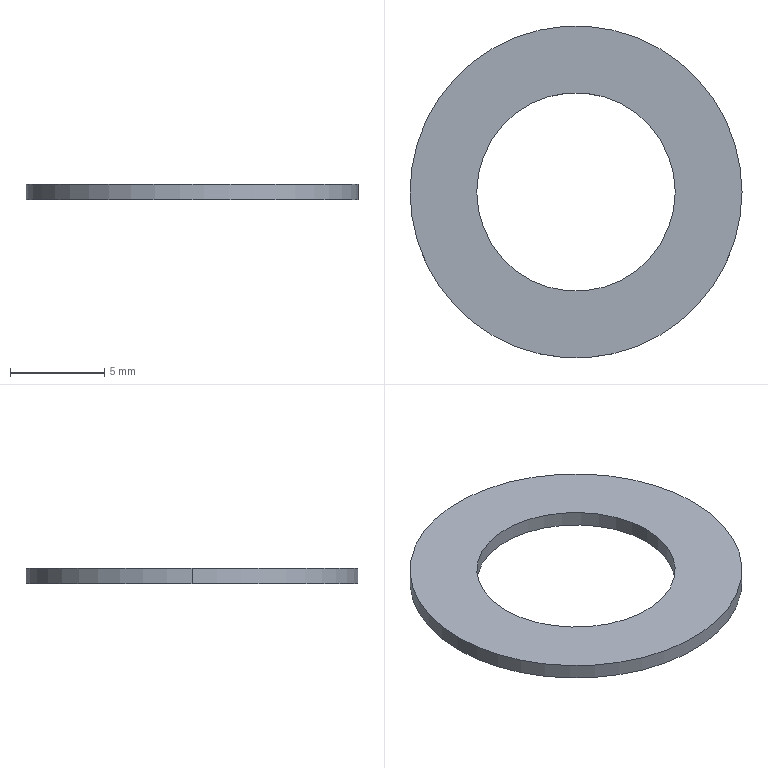Part | STEP file | 1 solid | 6 faces | box 17.57 x 17.57 x 0.8 mm | volume 124.693 mm3 | cylinder 4 | plane 2 | commonest cylinder face diameters 10.5 x2 17.57 x2
STEP:
#1=CARTESIAN_POINT('',(-5.25,0.,0.8));
#2=VERTEX_POINT('',#1);
#3=CARTESIAN_POINT('',(5.25,0.,0.8));
#4=VERTEX_POINT('',#3);
#5=CARTESIAN_POINT('',(0.,0.,0.8));
#6=DIRECTION('',(0.,0.,1.));
#7=DIRECTION('',(1.,0.,0.));
#8=AXIS2_PLACEMENT_3D('',#5,#6,#7);
#9=CIRCLE('',#8,5.25);
#10=EDGE_CURVE('',#2,#4,#9,.T.);
#11=ORIENTED_EDGE('',*,*,#10,.T.);
#12=CARTESIAN_POINT('',(5.25,0.,0.));
#13=VERTEX_POINT('',#12);
#14=CARTESIAN_POINT('',(5.25,0.,0.8));
#15=DIRECTION('',(0.,0.,-1.));
#16=VECTOR('',#15,1000.);
#17=LINE('',#14,#16);
#18=EDGE_CURVE('',#4,#13,#17,.T.);
#19=ORIENTED_EDGE('',*,*,#18,.T.);
#20=CARTESIAN_POINT('',(-5.25,0.,0.));
#21=VERTEX_POINT('',#20);
#22=CARTESIAN_POINT('',(0.,0.,0.));
#23=DIRECTION('',(0.,0.,1.));
#24=DIRECTION('',(1.,0.,0.));
#25=AXIS2_PLACEMENT_3D('',#22,#23,#24);
#26=CIRCLE('',#25,5.25);
#27=EDGE_CURVE('',#21,#13,#26,.T.);
#28=ORIENTED_EDGE('',*,*,#27,.F.);
#29=CARTESIAN_POINT('',(-5.25,0.,0.8));
#30=DIRECTION('',(0.,0.,-1.));
#31=VECTOR('',#30,1000.);
#32=LINE('',#29,#31);
#33=EDGE_CURVE('',#2,#21,#32,.T.);
#34=ORIENTED_EDGE('',*,*,#33,.F.);
#35=EDGE_LOOP('',(#11,#19,#28,#34));
#36=FACE_OUTER_BOUND('',#35,.T.);
#37=CARTESIAN_POINT('',(0.,0.,0.8));
#38=DIRECTION('',(0.,0.,-1.));
#39=DIRECTION('',(-1.,0.,0.));
#40=AXIS2_PLACEMENT_3D('',#37,#38,#39);
#41=CYLINDRICAL_SURFACE('',#40,5.25);
#42=ADVANCED_FACE('',(#36),#41,.F.);
#43=CARTESIAN_POINT('',(8.785,0.,0.8));
#44=VERTEX_POINT('',#43);
#45=CARTESIAN_POINT('',(-8.785,0.,0.8));
#46=VERTEX_POINT('',#45);
#47=CARTESIAN_POINT('',(0.,0.,0.8));
#48=DIRECTION('',(0.,0.,1.));
#49=DIRECTION('',(1.,0.,0.));
#50=AXIS2_PLACEMENT_3D('',#47,#48,#49);
#51=CIRCLE('',#50,8.785);
#52=EDGE_CURVE('',#44,#46,#51,.T.);
#53=ORIENTED_EDGE('',*,*,#52,.F.);
#54=CARTESIAN_POINT('',(8.785,0.,0.));
#55=VERTEX_POINT('',#54);
#56=CARTESIAN_POINT('',(8.785,0.,0.8));
#57=DIRECTION('',(0.,0.,-1.));
#58=VECTOR('',#57,1000.);
#59=LINE('',#56,#58);
#60=EDGE_CURVE('',#44,#55,#59,.T.);
#61=ORIENTED_EDGE('',*,*,#60,.T.);
#62=CARTESIAN_POINT('',(-8.785,0.,0.));
#63=VERTEX_POINT('',#62);
#64=CARTESIAN_POINT('',(0.,0.,0.));
#65=DIRECTION('',(0.,0.,1.));
#66=DIRECTION('',(1.,0.,0.));
#67=AXIS2_PLACEMENT_3D('',#64,#65,#66);
#68=CIRCLE('',#67,8.785);
#69=EDGE_CURVE('',#55,#63,#68,.T.);
#70=ORIENTED_EDGE('',*,*,#69,.T.);
#71=CARTESIAN_POINT('',(-8.785,0.,0.8));
#72=DIRECTION('',(0.,0.,-1.));
#73=VECTOR('',#72,1000.);
#74=LINE('',#71,#73);
#75=EDGE_CURVE('',#46,#63,#74,.T.);
#76=ORIENTED_EDGE('',*,*,#75,.F.);
#77=EDGE_LOOP('',(#53,#61,#70,#76));
#78=FACE_OUTER_BOUND('',#77,.T.);
#79=CARTESIAN_POINT('',(0.,0.,0.8));
#80=DIRECTION('',(0.,0.,-1.));
#81=DIRECTION('',(-1.,0.,0.));
#82=AXIS2_PLACEMENT_3D('',#79,#80,#81);
#83=CYLINDRICAL_SURFACE('',#82,8.785);
#84=ADVANCED_FACE('',(#78),#83,.T.);
#85=CARTESIAN_POINT('',(0.,0.,0.8));
#86=DIRECTION('',(0.,0.,1.));
#87=DIRECTION('',(1.,0.,0.));
#88=AXIS2_PLACEMENT_3D('',#85,#86,#87);
#89=CIRCLE('',#88,8.785);
#90=EDGE_CURVE('',#46,#44,#89,.T.);
#91=ORIENTED_EDGE('',*,*,#90,.T.);
#92=ORIENTED_EDGE('',*,*,#52,.T.);
#93=EDGE_LOOP('',(#91,#92));
#94=FACE_OUTER_BOUND('',#93,.T.);
#95=ORIENTED_EDGE('',*,*,#10,.F.);
#96=CARTESIAN_POINT('',(0.,0.,0.8));
#97=DIRECTION('',(0.,0.,1.));
#98=DIRECTION('',(1.,0.,0.));
#99=AXIS2_PLACEMENT_3D('',#96,#97,#98);
#100=CIRCLE('',#99,5.25);
#101=EDGE_CURVE('',#4,#2,#100,.T.);
#102=ORIENTED_EDGE('',*,*,#101,.F.);
#103=EDGE_LOOP('',(#95,#102));
#104=FACE_BOUND('',#103,.T.);
#105=CARTESIAN_POINT('',(0.,0.,0.8));
#106=DIRECTION('',(0.,0.,1.));
#107=DIRECTION('',(1.,0.,0.));
#108=AXIS2_PLACEMENT_3D('',#105,#106,#107);
#109=PLANE('',#108);
#110=ADVANCED_FACE('',(#94,#104),#109,.T.);
#111=CARTESIAN_POINT('',(0.,0.,0.));
#112=DIRECTION('',(0.,0.,1.));
#113=DIRECTION('',(1.,0.,0.));
#114=AXIS2_PLACEMENT_3D('',#111,#112,#113);
#115=CIRCLE('',#114,8.785);
#116=EDGE_CURVE('',#63,#55,#115,.T.);
#117=ORIENTED_EDGE('',*,*,#116,.F.);
#118=ORIENTED_EDGE('',*,*,#69,.F.);
#119=EDGE_LOOP('',(#117,#118));
#120=FACE_OUTER_BOUND('',#119,.T.);
#121=ORIENTED_EDGE('',*,*,#27,.T.);
#122=CARTESIAN_POINT('',(0.,0.,0.));
#123=DIRECTION('',(0.,0.,1.));
#124=DIRECTION('',(1.,0.,0.));
#125=AXIS2_PLACEMENT_3D('',#122,#123,#124);
#126=CIRCLE('',#125,5.25);
#127=EDGE_CURVE('',#13,#21,#126,.T.);
#128=ORIENTED_EDGE('',*,*,#127,.T.);
#129=EDGE_LOOP('',(#121,#128));
#130=FACE_BOUND('',#129,.T.);
#131=CARTESIAN_POINT('',(0.,0.,0.));
#132=DIRECTION('',(0.,0.,1.));
#133=DIRECTION('',(1.,0.,0.));
#134=AXIS2_PLACEMENT_3D('',#131,#132,#133);
#135=PLANE('',#134);
#136=ADVANCED_FACE('',(#120,#130),#135,.F.);
#137=ORIENTED_EDGE('',*,*,#60,.F.);
#138=ORIENTED_EDGE('',*,*,#90,.F.);
#139=ORIENTED_EDGE('',*,*,#75,.T.);
#140=ORIENTED_EDGE('',*,*,#116,.T.);
#141=EDGE_LOOP('',(#137,#138,#139,#140));
#142=FACE_OUTER_BOUND('',#141,.T.);
#143=CARTESIAN_POINT('',(0.,0.,0.8));
#144=DIRECTION('',(0.,0.,-1.));
#145=DIRECTION('',(-1.,0.,0.));
#146=AXIS2_PLACEMENT_3D('',#143,#144,#145);
#147=CYLINDRICAL_SURFACE('',#146,8.785);
#148=ADVANCED_FACE('',(#142),#147,.T.);
#149=ORIENTED_EDGE('',*,*,#18,.F.);
#150=ORIENTED_EDGE('',*,*,#101,.T.);
#151=ORIENTED_EDGE('',*,*,#33,.T.);
#152=ORIENTED_EDGE('',*,*,#127,.F.);
#153=EDGE_LOOP('',(#149,#150,#151,#152));
#154=FACE_OUTER_BOUND('',#153,.T.);
#155=CARTESIAN_POINT('',(0.,0.,0.8));
#156=DIRECTION('',(0.,0.,-1.));
#157=DIRECTION('',(-1.,0.,0.));
#158=AXIS2_PLACEMENT_3D('',#155,#156,#157);
#159=CYLINDRICAL_SURFACE('',#158,5.25);
#160=ADVANCED_FACE('',(#154),#159,.F.);
#161=CLOSED_SHELL('',(#42,#84,#110,#136,#148,#160));
#162=MANIFOLD_SOLID_BREP('',#161);
#163=CARTESIAN_POINT('',(0.,0.,0.));
#164=DIRECTION('',(0.,0.,1.));
#165=DIRECTION('',(1.,0.,0.));
#166=AXIS2_PLACEMENT_3D('',#163,#164,#165);
#167=(LENGTH_UNIT()NAMED_UNIT(*)SI_UNIT(.MILLI.,.METRE.));
#168=UNCERTAINTY_MEASURE_WITH_UNIT(LENGTH_MEASURE(0.00001),#167,'','');
#169=(NAMED_UNIT(*)PLANE_ANGLE_UNIT()SI_UNIT($,.RADIAN.));
#170=(NAMED_UNIT(*)SI_UNIT($,.STERADIAN.)SOLID_ANGLE_UNIT());
#171=(GEOMETRIC_REPRESENTATION_CONTEXT(3)GLOBAL_UNCERTAINTY_ASSIGNED_CONTEXT((#168))GLOBAL_UNIT_ASSIGNED_CONTEXT((#167,#169,#170))REPRESENTATION_CONTEXT('',''));
#172=ADVANCED_BREP_SHAPE_REPRESENTATION('',(#162,#166),#171);